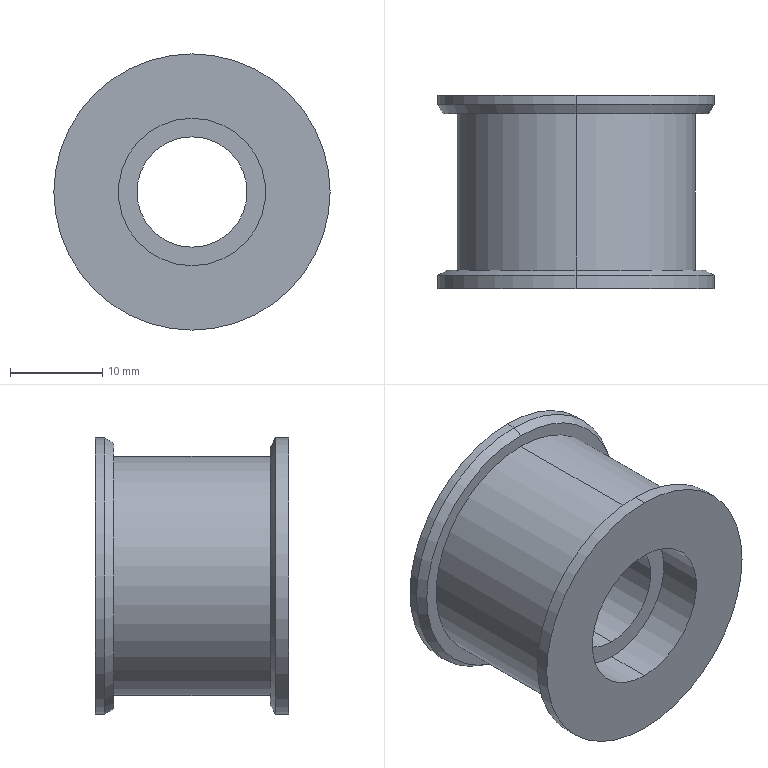Part | SolidWorks | features Chamfer 2, ICE 2, MirrorPattern 1, Revolution 1 | 1 solid | 22 faces | box 30 x 21 x 30 mm | volume 8531 mm3 | cylinder 12 | plane 6 | cone 4 | commonest cylinder face diameters 16 x4 30 x4 12 x2 25.98 x2
STEP:
#1=CARTESIAN_POINT('',(0.,-8.5,14.));
#2=VERTEX_POINT('',#1);
#3=CARTESIAN_POINT('',(0.,-8.5,-14.));
#4=VERTEX_POINT('',#3);
#5=CARTESIAN_POINT('',(0.,-8.5,0.));
#6=DIRECTION('',(0.,1.,0.));
#7=DIRECTION('',(0.,0.,-1.));
#8=AXIS2_PLACEMENT_3D('',#5,#6,#7);
#9=CIRCLE('',#8,14.);
#10=EDGE_CURVE('',#2,#4,#9,.T.);
#11=ORIENTED_EDGE('',*,*,#10,.F.);
#12=CARTESIAN_POINT('',(0.,-9.077,15.));
#13=VERTEX_POINT('',#12);
#14=CARTESIAN_POINT('',(0.,-9.077,15.));
#15=DIRECTION('',(0.,-0.5,0.866));
#16=VECTOR('',#15,1000.);
#17=LINE('',#14,#16);
#18=EDGE_CURVE('',#2,#13,#17,.T.);
#19=ORIENTED_EDGE('',*,*,#18,.T.);
#20=CARTESIAN_POINT('',(0.,-9.077,-15.));
#21=VERTEX_POINT('',#20);
#22=CARTESIAN_POINT('',(0.,-9.077,0.));
#23=DIRECTION('',(0.,-1.,0.));
#24=DIRECTION('',(0.,0.,-1.));
#25=AXIS2_PLACEMENT_3D('',#22,#23,#24);
#26=CIRCLE('',#25,15.);
#27=EDGE_CURVE('',#21,#13,#26,.T.);
#28=ORIENTED_EDGE('',*,*,#27,.F.);
#29=CARTESIAN_POINT('',(0.,-9.077,-15.));
#30=DIRECTION('',(0.,-0.5,-0.866));
#31=VECTOR('',#30,1000.);
#32=LINE('',#29,#31);
#33=EDGE_CURVE('',#4,#21,#32,.T.);
#34=ORIENTED_EDGE('',*,*,#33,.F.);
#35=EDGE_LOOP('',(#11,#19,#28,#34));
#36=FACE_OUTER_BOUND('',#35,.T.);
#37=CARTESIAN_POINT('',(0.,-9.077,0.));
#38=DIRECTION('',(0.,-1.,0.));
#39=DIRECTION('',(0.,0.,-1.));
#40=AXIS2_PLACEMENT_3D('',#37,#38,#39);
#41=CONICAL_SURFACE('',#40,15.,1.047);
#42=ADVANCED_FACE('',(#36),#41,.T.);
#43=CARTESIAN_POINT('',(0.,8.5,-14.423));
#44=VERTEX_POINT('',#43);
#45=CARTESIAN_POINT('',(0.,8.5,14.423));
#46=VERTEX_POINT('',#45);
#47=CARTESIAN_POINT('',(0.,8.5,0.));
#48=DIRECTION('',(0.,-1.,0.));
#49=DIRECTION('',(0.,0.,1.));
#50=AXIS2_PLACEMENT_3D('',#47,#48,#49);
#51=CIRCLE('',#50,14.423);
#52=EDGE_CURVE('',#44,#46,#51,.T.);
#53=ORIENTED_EDGE('',*,*,#52,.F.);
#54=CARTESIAN_POINT('',(0.,9.5,-15.));
#55=VERTEX_POINT('',#54);
#56=CARTESIAN_POINT('',(0.,8.5,-14.423));
#57=DIRECTION('',(0.,0.866,-0.5));
#58=VECTOR('',#57,1000.);
#59=LINE('',#56,#58);
#60=EDGE_CURVE('',#44,#55,#59,.T.);
#61=ORIENTED_EDGE('',*,*,#60,.T.);
#62=CARTESIAN_POINT('',(0.,9.5,15.));
#63=VERTEX_POINT('',#62);
#64=CARTESIAN_POINT('',(0.,9.5,0.));
#65=DIRECTION('',(0.,1.,0.));
#66=DIRECTION('',(0.,0.,1.));
#67=AXIS2_PLACEMENT_3D('',#64,#65,#66);
#68=CIRCLE('',#67,15.);
#69=EDGE_CURVE('',#63,#55,#68,.T.);
#70=ORIENTED_EDGE('',*,*,#69,.F.);
#71=CARTESIAN_POINT('',(0.,8.5,14.423));
#72=DIRECTION('',(0.,0.866,0.5));
#73=VECTOR('',#72,1000.);
#74=LINE('',#71,#73);
#75=EDGE_CURVE('',#46,#63,#74,.T.);
#76=ORIENTED_EDGE('',*,*,#75,.F.);
#77=EDGE_LOOP('',(#53,#61,#70,#76));
#78=FACE_OUTER_BOUND('',#77,.T.);
#79=CARTESIAN_POINT('',(0.,8.5,0.));
#80=DIRECTION('',(0.,1.,0.));
#81=DIRECTION('',(0.,0.,1.));
#82=AXIS2_PLACEMENT_3D('',#79,#80,#81);
#83=CONICAL_SURFACE('',#82,14.423,0.5236);
#84=ADVANCED_FACE('',(#78),#83,.T.);
#85=ORIENTED_EDGE('',*,*,#69,.T.);
#86=CARTESIAN_POINT('',(0.,10.5,-15.));
#87=VERTEX_POINT('',#86);
#88=CARTESIAN_POINT('',(0.,8.5,-15.));
#89=DIRECTION('',(0.,1.,0.));
#90=VECTOR('',#89,1000.);
#91=LINE('',#88,#90);
#92=EDGE_CURVE('',#55,#87,#91,.T.);
#93=ORIENTED_EDGE('',*,*,#92,.T.);
#94=CARTESIAN_POINT('',(0.,10.5,15.));
#95=VERTEX_POINT('',#94);
#96=CARTESIAN_POINT('',(0.,10.5,0.));
#97=DIRECTION('',(0.,-1.,0.));
#98=DIRECTION('',(0.,0.,-1.));
#99=AXIS2_PLACEMENT_3D('',#96,#97,#98);
#100=CIRCLE('',#99,15.);
#101=EDGE_CURVE('',#87,#95,#100,.T.);
#102=ORIENTED_EDGE('',*,*,#101,.T.);
#103=CARTESIAN_POINT('',(0.,8.5,15.));
#104=DIRECTION('',(0.,1.,0.));
#105=VECTOR('',#104,1000.);
#106=LINE('',#103,#105);
#107=EDGE_CURVE('',#63,#95,#106,.T.);
#108=ORIENTED_EDGE('',*,*,#107,.F.);
#109=EDGE_LOOP('',(#85,#93,#102,#108));
#110=FACE_OUTER_BOUND('',#109,.T.);
#111=CARTESIAN_POINT('',(0.,8.5,0.));
#112=DIRECTION('',(0.,1.,0.));
#113=DIRECTION('',(0.,0.,1.));
#114=AXIS2_PLACEMENT_3D('',#111,#112,#113);
#115=CYLINDRICAL_SURFACE('',#114,15.);
#116=ADVANCED_FACE('',(#110),#115,.T.);
#117=CARTESIAN_POINT('',(0.,5.5,8.));
#118=VERTEX_POINT('',#117);
#119=CARTESIAN_POINT('',(0.,5.5,-8.));
#120=VERTEX_POINT('',#119);
#121=CARTESIAN_POINT('',(0.,5.5,0.));
#122=DIRECTION('',(0.,-1.,0.));
#123=DIRECTION('',(0.,0.,-1.));
#124=AXIS2_PLACEMENT_3D('',#121,#122,#123);
#125=CIRCLE('',#124,8.);
#126=EDGE_CURVE('',#118,#120,#125,.T.);
#127=ORIENTED_EDGE('',*,*,#126,.T.);
#128=CARTESIAN_POINT('',(0.,10.5,-8.));
#129=VERTEX_POINT('',#128);
#130=CARTESIAN_POINT('',(0.,5.5,-8.));
#131=DIRECTION('',(0.,1.,0.));
#132=VECTOR('',#131,1000.);
#133=LINE('',#130,#132);
#134=EDGE_CURVE('',#120,#129,#133,.T.);
#135=ORIENTED_EDGE('',*,*,#134,.T.);
#136=CARTESIAN_POINT('',(0.,10.5,8.));
#137=VERTEX_POINT('',#136);
#138=CARTESIAN_POINT('',(0.,10.5,0.));
#139=DIRECTION('',(0.,-1.,0.));
#140=DIRECTION('',(0.,0.,-1.));
#141=AXIS2_PLACEMENT_3D('',#138,#139,#140);
#142=CIRCLE('',#141,8.);
#143=EDGE_CURVE('',#137,#129,#142,.T.);
#144=ORIENTED_EDGE('',*,*,#143,.F.);
#145=CARTESIAN_POINT('',(0.,5.5,8.));
#146=DIRECTION('',(0.,1.,0.));
#147=VECTOR('',#146,1000.);
#148=LINE('',#145,#147);
#149=EDGE_CURVE('',#118,#137,#148,.T.);
#150=ORIENTED_EDGE('',*,*,#149,.F.);
#151=EDGE_LOOP('',(#127,#135,#144,#150));
#152=FACE_OUTER_BOUND('',#151,.T.);
#153=CARTESIAN_POINT('',(0.,5.5,0.));
#154=DIRECTION('',(0.,1.,0.));
#155=DIRECTION('',(0.,0.,1.));
#156=AXIS2_PLACEMENT_3D('',#153,#154,#155);
#157=CYLINDRICAL_SURFACE('',#156,8.);
#158=ADVANCED_FACE('',(#152),#157,.F.);
#159=ORIENTED_EDGE('',*,*,#27,.T.);
#160=CARTESIAN_POINT('',(0.,-10.5,15.));
#161=VERTEX_POINT('',#160);
#162=CARTESIAN_POINT('',(0.,-8.5,15.));
#163=DIRECTION('',(0.,-1.,0.));
#164=VECTOR('',#163,1000.);
#165=LINE('',#162,#164);
#166=EDGE_CURVE('',#13,#161,#165,.T.);
#167=ORIENTED_EDGE('',*,*,#166,.T.);
#168=CARTESIAN_POINT('',(0.,-10.5,-15.));
#169=VERTEX_POINT('',#168);
#170=CARTESIAN_POINT('',(0.,-10.5,0.));
#171=DIRECTION('',(0.,-1.,0.));
#172=DIRECTION('',(0.,0.,-1.));
#173=AXIS2_PLACEMENT_3D('',#170,#171,#172);
#174=CIRCLE('',#173,15.);
#175=EDGE_CURVE('',#169,#161,#174,.T.);
#176=ORIENTED_EDGE('',*,*,#175,.F.);
#177=CARTESIAN_POINT('',(0.,-8.5,-15.));
#178=DIRECTION('',(0.,-1.,0.));
#179=VECTOR('',#178,1000.);
#180=LINE('',#177,#179);
#181=EDGE_CURVE('',#21,#169,#180,.T.);
#182=ORIENTED_EDGE('',*,*,#181,.F.);
#183=EDGE_LOOP('',(#159,#167,#176,#182));
#184=FACE_OUTER_BOUND('',#183,.T.);
#185=CARTESIAN_POINT('',(0.,-8.5,0.));
#186=DIRECTION('',(0.,-1.,0.));
#187=DIRECTION('',(0.,0.,-1.));
#188=AXIS2_PLACEMENT_3D('',#185,#186,#187);
#189=CYLINDRICAL_SURFACE('',#188,15.);
#190=ADVANCED_FACE('',(#184),#189,.T.);
#191=CARTESIAN_POINT('',(0.,-5.5,8.));
#192=VERTEX_POINT('',#191);
#193=CARTESIAN_POINT('',(0.,-5.5,-8.));
#194=VERTEX_POINT('',#193);
#195=CARTESIAN_POINT('',(0.,-5.5,0.));
#196=DIRECTION('',(0.,-1.,0.));
#197=DIRECTION('',(0.,0.,-1.));
#198=AXIS2_PLACEMENT_3D('',#195,#196,#197);
#199=CIRCLE('',#198,8.);
#200=EDGE_CURVE('',#192,#194,#199,.T.);
#201=ORIENTED_EDGE('',*,*,#200,.F.);
#202=CARTESIAN_POINT('',(0.,-10.5,8.));
#203=VERTEX_POINT('',#202);
#204=CARTESIAN_POINT('',(0.,-5.5,8.));
#205=DIRECTION('',(0.,-1.,0.));
#206=VECTOR('',#205,1000.);
#207=LINE('',#204,#206);
#208=EDGE_CURVE('',#192,#203,#207,.T.);
#209=ORIENTED_EDGE('',*,*,#208,.T.);
#210=CARTESIAN_POINT('',(0.,-10.5,-8.));
#211=VERTEX_POINT('',#210);
#212=CARTESIAN_POINT('',(0.,-10.5,0.));
#213=DIRECTION('',(0.,-1.,0.));
#214=DIRECTION('',(0.,0.,-1.));
#215=AXIS2_PLACEMENT_3D('',#212,#213,#214);
#216=CIRCLE('',#215,8.);
#217=EDGE_CURVE('',#203,#211,#216,.T.);
#218=ORIENTED_EDGE('',*,*,#217,.T.);
#219=CARTESIAN_POINT('',(0.,-5.5,-8.));
#220=DIRECTION('',(0.,-1.,0.));
#221=VECTOR('',#220,1000.);
#222=LINE('',#219,#221);
#223=EDGE_CURVE('',#194,#211,#222,.T.);
#224=ORIENTED_EDGE('',*,*,#223,.F.);
#225=EDGE_LOOP('',(#201,#209,#218,#224));
#226=FACE_OUTER_BOUND('',#225,.T.);
#227=CARTESIAN_POINT('',(0.,-5.5,0.));
#228=DIRECTION('',(0.,-1.,0.));
#229=DIRECTION('',(0.,0.,-1.));
#230=AXIS2_PLACEMENT_3D('',#227,#228,#229);
#231=CYLINDRICAL_SURFACE('',#230,8.);
#232=ADVANCED_FACE('',(#226),#231,.F.);
#233=CARTESIAN_POINT('',(0.,5.5,-6.));
#234=VERTEX_POINT('',#233);
#235=CARTESIAN_POINT('',(0.,5.5,6.));
#236=VERTEX_POINT('',#235);
#237=CARTESIAN_POINT('',(0.,5.5,0.));
#238=DIRECTION('',(0.,1.,0.));
#239=DIRECTION('',(0.,0.,1.));
#240=AXIS2_PLACEMENT_3D('',#237,#238,#239);
#241=CIRCLE('',#240,6.);
#242=EDGE_CURVE('',#234,#236,#241,.T.);
#243=ORIENTED_EDGE('',*,*,#242,.T.);
#244=CARTESIAN_POINT('',(0.,-5.5,6.));
#245=VERTEX_POINT('',#244);
#246=CARTESIAN_POINT('',(0.,0.,6.));
#247=DIRECTION('',(0.,-1.,0.));
#248=VECTOR('',#247,1000.);
#249=LINE('',#246,#248);
#250=EDGE_CURVE('',#236,#245,#249,.T.);
#251=ORIENTED_EDGE('',*,*,#250,.T.);
#252=CARTESIAN_POINT('',(0.,-5.5,-6.));
#253=VERTEX_POINT('',#252);
#254=CARTESIAN_POINT('',(0.,-5.5,0.));
#255=DIRECTION('',(0.,-1.,0.));
#256=DIRECTION('',(0.,0.,-1.));
#257=AXIS2_PLACEMENT_3D('',#254,#255,#256);
#258=CIRCLE('',#257,6.);
#259=EDGE_CURVE('',#245,#253,#258,.T.);
#260=ORIENTED_EDGE('',*,*,#259,.T.);
#261=CARTESIAN_POINT('',(0.,0.,-6.));
#262=DIRECTION('',(0.,-1.,0.));
#263=VECTOR('',#262,1000.);
#264=LINE('',#261,#263);
#265=EDGE_CURVE('',#234,#253,#264,.T.);
#266=ORIENTED_EDGE('',*,*,#265,.F.);
#267=EDGE_LOOP('',(#243,#251,#260,#266));
#268=FACE_OUTER_BOUND('',#267,.T.);
#269=CARTESIAN_POINT('',(0.,0.,0.));
#270=DIRECTION('',(0.,-1.,0.));
#271=DIRECTION('',(0.,0.,-1.));
#272=AXIS2_PLACEMENT_3D('',#269,#270,#271);
#273=CYLINDRICAL_SURFACE('',#272,6.);
#274=ADVANCED_FACE('',(#268),#273,.F.);
#275=CARTESIAN_POINT('',(0.,8.5,-12.99));
#276=VERTEX_POINT('',#275);
#277=CARTESIAN_POINT('',(0.,8.5,12.99));
#278=VERTEX_POINT('',#277);
#279=CARTESIAN_POINT('',(0.,8.5,0.));
#280=DIRECTION('',(0.,-1.,0.));
#281=DIRECTION('',(0.,0.,1.));
#282=AXIS2_PLACEMENT_3D('',#279,#280,#281);
#283=CIRCLE('',#282,12.99);
#284=EDGE_CURVE('',#276,#278,#283,.T.);
#285=ORIENTED_EDGE('',*,*,#284,.T.);
#286=CARTESIAN_POINT('',(0.,-8.5,12.99));
#287=VERTEX_POINT('',#286);
#288=CARTESIAN_POINT('',(0.,0.,12.99));
#289=DIRECTION('',(0.,-1.,0.));
#290=VECTOR('',#289,1000.);
#291=LINE('',#288,#290);
#292=EDGE_CURVE('',#278,#287,#291,.T.);
#293=ORIENTED_EDGE('',*,*,#292,.T.);
#294=CARTESIAN_POINT('',(0.,-8.5,-12.99));
#295=VERTEX_POINT('',#294);
#296=CARTESIAN_POINT('',(0.,-8.5,0.));
#297=DIRECTION('',(0.,1.,0.));
#298=DIRECTION('',(0.,0.,-1.));
#299=AXIS2_PLACEMENT_3D('',#296,#297,#298);
#300=CIRCLE('',#299,12.99);
#301=EDGE_CURVE('',#287,#295,#300,.T.);
#302=ORIENTED_EDGE('',*,*,#301,.T.);
#303=CARTESIAN_POINT('',(0.,0.,-12.99));
#304=DIRECTION('',(0.,-1.,0.));
#305=VECTOR('',#304,1000.);
#306=LINE('',#303,#305);
#307=EDGE_CURVE('',#276,#295,#306,.T.);
#308=ORIENTED_EDGE('',*,*,#307,.F.);
#309=EDGE_LOOP('',(#285,#293,#302,#308));
#310=FACE_OUTER_BOUND('',#309,.T.);
#311=CARTESIAN_POINT('',(0.,0.,0.));
#312=DIRECTION('',(0.,-1.,0.));
#313=DIRECTION('',(0.,0.,-1.));
#314=AXIS2_PLACEMENT_3D('',#311,#312,#313);
#315=CYLINDRICAL_SURFACE('',#314,12.99);
#316=ADVANCED_FACE('',(#310),#315,.T.);
#317=ORIENTED_EDGE('',*,*,#292,.F.);
#318=CARTESIAN_POINT('',(0.,8.5,0.));
#319=DIRECTION('',(0.,-1.,0.));
#320=DIRECTION('',(0.,0.,1.));
#321=AXIS2_PLACEMENT_3D('',#318,#319,#320);
#322=CIRCLE('',#321,12.99);
#323=EDGE_CURVE('',#278,#276,#322,.T.);
#324=ORIENTED_EDGE('',*,*,#323,.T.);
#325=ORIENTED_EDGE('',*,*,#307,.T.);
#326=CARTESIAN_POINT('',(0.,-8.5,0.));
#327=DIRECTION('',(0.,1.,0.));
#328=DIRECTION('',(0.,0.,-1.));
#329=AXIS2_PLACEMENT_3D('',#326,#327,#328);
#330=CIRCLE('',#329,12.99);
#331=EDGE_CURVE('',#295,#287,#330,.T.);
#332=ORIENTED_EDGE('',*,*,#331,.T.);
#333=EDGE_LOOP('',(#317,#324,#325,#332));
#334=FACE_OUTER_BOUND('',#333,.T.);
#335=CARTESIAN_POINT('',(0.,0.,0.));
#336=DIRECTION('',(0.,-1.,0.));
#337=DIRECTION('',(0.,0.,-1.));
#338=AXIS2_PLACEMENT_3D('',#335,#336,#337);
#339=CYLINDRICAL_SURFACE('',#338,12.99);
#340=ADVANCED_FACE('',(#334),#339,.T.);
#341=ORIENTED_EDGE('',*,*,#250,.F.);
#342=CARTESIAN_POINT('',(0.,5.5,0.));
#343=DIRECTION('',(0.,1.,0.));
#344=DIRECTION('',(0.,0.,1.));
#345=AXIS2_PLACEMENT_3D('',#342,#343,#344);
#346=CIRCLE('',#345,6.);
#347=EDGE_CURVE('',#236,#234,#346,.T.);
#348=ORIENTED_EDGE('',*,*,#347,.T.);
#349=ORIENTED_EDGE('',*,*,#265,.T.);
#350=CARTESIAN_POINT('',(0.,-5.5,0.));
#351=DIRECTION('',(0.,-1.,0.));
#352=DIRECTION('',(0.,0.,-1.));
#353=AXIS2_PLACEMENT_3D('',#350,#351,#352);
#354=CIRCLE('',#353,6.);
#355=EDGE_CURVE('',#253,#245,#354,.T.);
#356=ORIENTED_EDGE('',*,*,#355,.T.);
#357=EDGE_LOOP('',(#341,#348,#349,#356));
#358=FACE_OUTER_BOUND('',#357,.T.);
#359=CARTESIAN_POINT('',(0.,0.,0.));
#360=DIRECTION('',(0.,-1.,0.));
#361=DIRECTION('',(0.,0.,-1.));
#362=AXIS2_PLACEMENT_3D('',#359,#360,#361);
#363=CYLINDRICAL_SURFACE('',#362,6.);
#364=ADVANCED_FACE('',(#358),#363,.F.);
#365=ORIENTED_EDGE('',*,*,#143,.T.);
#366=CARTESIAN_POINT('',(0.,10.5,0.));
#367=DIRECTION('',(0.,-1.,0.));
#368=DIRECTION('',(0.,0.,-1.));
#369=AXIS2_PLACEMENT_3D('',#366,#367,#368);
#370=CIRCLE('',#369,8.);
#371=EDGE_CURVE('',#129,#137,#370,.T.);
#372=ORIENTED_EDGE('',*,*,#371,.T.);
#373=EDGE_LOOP('',(#365,#372));
#374=FACE_BOUND('',#373,.T.);
#375=CARTESIAN_POINT('',(0.,10.5,0.));
#376=DIRECTION('',(0.,-1.,0.));
#377=DIRECTION('',(0.,0.,-1.));
#378=AXIS2_PLACEMENT_3D('',#375,#376,#377);
#379=CIRCLE('',#378,15.);
#380=EDGE_CURVE('',#95,#87,#379,.T.);
#381=ORIENTED_EDGE('',*,*,#380,.F.);
#382=ORIENTED_EDGE('',*,*,#101,.F.);
#383=EDGE_LOOP('',(#381,#382));
#384=FACE_OUTER_BOUND('',#383,.T.);
#385=CARTESIAN_POINT('',(6.,10.5,0.));
#386=DIRECTION('',(0.,1.,0.));
#387=DIRECTION('',(0.,0.,1.));
#388=AXIS2_PLACEMENT_3D('',#385,#386,#387);
#389=PLANE('',#388);
#390=ADVANCED_FACE('',(#374,#384),#389,.T.);
#391=CARTESIAN_POINT('',(0.,-10.5,0.));
#392=DIRECTION('',(0.,-1.,0.));
#393=DIRECTION('',(0.,0.,-1.));
#394=AXIS2_PLACEMENT_3D('',#391,#392,#393);
#395=CIRCLE('',#394,8.);
#396=EDGE_CURVE('',#211,#203,#395,.T.);
#397=ORIENTED_EDGE('',*,*,#396,.F.);
#398=ORIENTED_EDGE('',*,*,#217,.F.);
#399=EDGE_LOOP('',(#397,#398));
#400=FACE_BOUND('',#399,.T.);
#401=ORIENTED_EDGE('',*,*,#175,.T.);
#402=CARTESIAN_POINT('',(0.,-10.5,0.));
#403=DIRECTION('',(0.,-1.,0.));
#404=DIRECTION('',(0.,0.,-1.));
#405=AXIS2_PLACEMENT_3D('',#402,#403,#404);
#406=CIRCLE('',#405,15.);
#407=EDGE_CURVE('',#161,#169,#406,.T.);
#408=ORIENTED_EDGE('',*,*,#407,.T.);
#409=EDGE_LOOP('',(#401,#408));
#410=FACE_OUTER_BOUND('',#409,.T.);
#411=CARTESIAN_POINT('',(12.99,-10.5,0.));
#412=DIRECTION('',(0.,-1.,0.));
#413=DIRECTION('',(0.,0.,-1.));
#414=AXIS2_PLACEMENT_3D('',#411,#412,#413);
#415=PLANE('',#414);
#416=ADVANCED_FACE('',(#400,#410),#415,.T.);
#417=ORIENTED_EDGE('',*,*,#208,.F.);
#418=CARTESIAN_POINT('',(0.,-5.5,0.));
#419=DIRECTION('',(0.,-1.,0.));
#420=DIRECTION('',(0.,0.,-1.));
#421=AXIS2_PLACEMENT_3D('',#418,#419,#420);
#422=CIRCLE('',#421,8.);
#423=EDGE_CURVE('',#194,#192,#422,.T.);
#424=ORIENTED_EDGE('',*,*,#423,.F.);
#425=ORIENTED_EDGE('',*,*,#223,.T.);
#426=ORIENTED_EDGE('',*,*,#396,.T.);
#427=EDGE_LOOP('',(#417,#424,#425,#426));
#428=FACE_OUTER_BOUND('',#427,.T.);
#429=CARTESIAN_POINT('',(0.,-5.5,0.));
#430=DIRECTION('',(0.,-1.,0.));
#431=DIRECTION('',(0.,0.,-1.));
#432=AXIS2_PLACEMENT_3D('',#429,#430,#431);
#433=CYLINDRICAL_SURFACE('',#432,8.);
#434=ADVANCED_FACE('',(#428),#433,.F.);
#435=ORIENTED_EDGE('',*,*,#355,.F.);
#436=ORIENTED_EDGE('',*,*,#259,.F.);
#437=EDGE_LOOP('',(#435,#436));
#438=FACE_BOUND('',#437,.T.);
#439=ORIENTED_EDGE('',*,*,#423,.T.);
#440=ORIENTED_EDGE('',*,*,#200,.T.);
#441=EDGE_LOOP('',(#439,#440));
#442=FACE_OUTER_BOUND('',#441,.T.);
#443=CARTESIAN_POINT('',(0.,-5.5,0.));
#444=DIRECTION('',(0.,-1.,0.));
#445=DIRECTION('',(0.,0.,-1.));
#446=AXIS2_PLACEMENT_3D('',#443,#444,#445);
#447=PLANE('',#446);
#448=ADVANCED_FACE('',(#438,#442),#447,.T.);
#449=ORIENTED_EDGE('',*,*,#166,.F.);
#450=CARTESIAN_POINT('',(0.,-9.077,0.));
#451=DIRECTION('',(0.,-1.,0.));
#452=DIRECTION('',(0.,0.,-1.));
#453=AXIS2_PLACEMENT_3D('',#450,#451,#452);
#454=CIRCLE('',#453,15.);
#455=EDGE_CURVE('',#13,#21,#454,.T.);
#456=ORIENTED_EDGE('',*,*,#455,.T.);
#457=ORIENTED_EDGE('',*,*,#181,.T.);
#458=ORIENTED_EDGE('',*,*,#407,.F.);
#459=EDGE_LOOP('',(#449,#456,#457,#458));
#460=FACE_OUTER_BOUND('',#459,.T.);
#461=CARTESIAN_POINT('',(0.,-8.5,0.));
#462=DIRECTION('',(0.,-1.,0.));
#463=DIRECTION('',(0.,0.,-1.));
#464=AXIS2_PLACEMENT_3D('',#461,#462,#463);
#465=CYLINDRICAL_SURFACE('',#464,15.);
#466=ADVANCED_FACE('',(#460),#465,.T.);
#467=CARTESIAN_POINT('',(0.,-8.5,0.));
#468=DIRECTION('',(0.,1.,0.));
#469=DIRECTION('',(0.,0.,-1.));
#470=AXIS2_PLACEMENT_3D('',#467,#468,#469);
#471=CIRCLE('',#470,14.);
#472=EDGE_CURVE('',#4,#2,#471,.T.);
#473=ORIENTED_EDGE('',*,*,#472,.T.);
#474=ORIENTED_EDGE('',*,*,#10,.T.);
#475=EDGE_LOOP('',(#473,#474));
#476=FACE_OUTER_BOUND('',#475,.T.);
#477=ORIENTED_EDGE('',*,*,#331,.F.);
#478=ORIENTED_EDGE('',*,*,#301,.F.);
#479=EDGE_LOOP('',(#477,#478));
#480=FACE_BOUND('',#479,.T.);
#481=CARTESIAN_POINT('',(0.,-8.5,0.));
#482=DIRECTION('',(0.,-1.,0.));
#483=DIRECTION('',(0.,0.,-1.));
#484=AXIS2_PLACEMENT_3D('',#481,#482,#483);
#485=PLANE('',#484);
#486=ADVANCED_FACE('',(#476,#480),#485,.F.);
#487=ORIENTED_EDGE('',*,*,#134,.F.);
#488=CARTESIAN_POINT('',(0.,5.5,0.));
#489=DIRECTION('',(0.,-1.,0.));
#490=DIRECTION('',(0.,0.,-1.));
#491=AXIS2_PLACEMENT_3D('',#488,#489,#490);
#492=CIRCLE('',#491,8.);
#493=EDGE_CURVE('',#120,#118,#492,.T.);
#494=ORIENTED_EDGE('',*,*,#493,.T.);
#495=ORIENTED_EDGE('',*,*,#149,.T.);
#496=ORIENTED_EDGE('',*,*,#371,.F.);
#497=EDGE_LOOP('',(#487,#494,#495,#496));
#498=FACE_OUTER_BOUND('',#497,.T.);
#499=CARTESIAN_POINT('',(0.,5.5,0.));
#500=DIRECTION('',(0.,1.,0.));
#501=DIRECTION('',(0.,0.,1.));
#502=AXIS2_PLACEMENT_3D('',#499,#500,#501);
#503=CYLINDRICAL_SURFACE('',#502,8.);
#504=ADVANCED_FACE('',(#498),#503,.F.);
#505=ORIENTED_EDGE('',*,*,#242,.F.);
#506=ORIENTED_EDGE('',*,*,#347,.F.);
#507=EDGE_LOOP('',(#505,#506));
#508=FACE_BOUND('',#507,.T.);
#509=ORIENTED_EDGE('',*,*,#126,.F.);
#510=ORIENTED_EDGE('',*,*,#493,.F.);
#511=EDGE_LOOP('',(#509,#510));
#512=FACE_OUTER_BOUND('',#511,.T.);
#513=CARTESIAN_POINT('',(0.,5.5,0.));
#514=DIRECTION('',(0.,1.,0.));
#515=DIRECTION('',(0.,0.,-1.));
#516=AXIS2_PLACEMENT_3D('',#513,#514,#515);
#517=PLANE('',#516);
#518=ADVANCED_FACE('',(#508,#512),#517,.T.);
#519=CARTESIAN_POINT('',(0.,8.5,0.));
#520=DIRECTION('',(0.,-1.,0.));
#521=DIRECTION('',(0.,0.,1.));
#522=AXIS2_PLACEMENT_3D('',#519,#520,#521);
#523=CIRCLE('',#522,14.423);
#524=EDGE_CURVE('',#46,#44,#523,.T.);
#525=ORIENTED_EDGE('',*,*,#524,.T.);
#526=ORIENTED_EDGE('',*,*,#52,.T.);
#527=EDGE_LOOP('',(#525,#526));
#528=FACE_OUTER_BOUND('',#527,.T.);
#529=ORIENTED_EDGE('',*,*,#284,.F.);
#530=ORIENTED_EDGE('',*,*,#323,.F.);
#531=EDGE_LOOP('',(#529,#530));
#532=FACE_BOUND('',#531,.T.);
#533=CARTESIAN_POINT('',(0.,8.5,0.));
#534=DIRECTION('',(0.,1.,0.));
#535=DIRECTION('',(0.,0.,-1.));
#536=AXIS2_PLACEMENT_3D('',#533,#534,#535);
#537=PLANE('',#536);
#538=ADVANCED_FACE('',(#528,#532),#537,.F.);
#539=ORIENTED_EDGE('',*,*,#92,.F.);
#540=CARTESIAN_POINT('',(0.,9.5,0.));
#541=DIRECTION('',(0.,1.,0.));
#542=DIRECTION('',(0.,0.,1.));
#543=AXIS2_PLACEMENT_3D('',#540,#541,#542);
#544=CIRCLE('',#543,15.);
#545=EDGE_CURVE('',#55,#63,#544,.T.);
#546=ORIENTED_EDGE('',*,*,#545,.T.);
#547=ORIENTED_EDGE('',*,*,#107,.T.);
#548=ORIENTED_EDGE('',*,*,#380,.T.);
#549=EDGE_LOOP('',(#539,#546,#547,#548));
#550=FACE_OUTER_BOUND('',#549,.T.);
#551=CARTESIAN_POINT('',(0.,8.5,0.));
#552=DIRECTION('',(0.,1.,0.));
#553=DIRECTION('',(0.,0.,1.));
#554=AXIS2_PLACEMENT_3D('',#551,#552,#553);
#555=CYLINDRICAL_SURFACE('',#554,15.);
#556=ADVANCED_FACE('',(#550),#555,.T.);
#557=ORIENTED_EDGE('',*,*,#60,.F.);
#558=ORIENTED_EDGE('',*,*,#524,.F.);
#559=ORIENTED_EDGE('',*,*,#75,.T.);
#560=ORIENTED_EDGE('',*,*,#545,.F.);
#561=EDGE_LOOP('',(#557,#558,#559,#560));
#562=FACE_OUTER_BOUND('',#561,.T.);
#563=CARTESIAN_POINT('',(0.,8.5,0.));
#564=DIRECTION('',(0.,1.,0.));
#565=DIRECTION('',(0.,0.,1.));
#566=AXIS2_PLACEMENT_3D('',#563,#564,#565);
#567=CONICAL_SURFACE('',#566,14.423,0.5236);
#568=ADVANCED_FACE('',(#562),#567,.T.);
#569=ORIENTED_EDGE('',*,*,#18,.F.);
#570=ORIENTED_EDGE('',*,*,#472,.F.);
#571=ORIENTED_EDGE('',*,*,#33,.T.);
#572=ORIENTED_EDGE('',*,*,#455,.F.);
#573=EDGE_LOOP('',(#569,#570,#571,#572));
#574=FACE_OUTER_BOUND('',#573,.T.);
#575=CARTESIAN_POINT('',(0.,-9.077,0.));
#576=DIRECTION('',(0.,-1.,0.));
#577=DIRECTION('',(0.,0.,-1.));
#578=AXIS2_PLACEMENT_3D('',#575,#576,#577);
#579=CONICAL_SURFACE('',#578,15.,1.047);
#580=ADVANCED_FACE('',(#574),#579,.T.);
#581=CLOSED_SHELL('',(#42,#84,#116,#158,#190,#232,#274,#316,#340,#364,#390,#416,#434,#448,#466,#486,#504,#518,#538,#556,#568,#580));
#582=MANIFOLD_SOLID_BREP('',#581);
#583=CARTESIAN_POINT('',(0.,0.,0.));
#584=DIRECTION('',(0.,0.,1.));
#585=DIRECTION('',(1.,0.,0.));
#586=AXIS2_PLACEMENT_3D('',#583,#584,#585);
#587=(LENGTH_UNIT()NAMED_UNIT(*)SI_UNIT(.MILLI.,.METRE.));
#588=UNCERTAINTY_MEASURE_WITH_UNIT(LENGTH_MEASURE(0.00001),#587,'','');
#589=(NAMED_UNIT(*)PLANE_ANGLE_UNIT()SI_UNIT($,.RADIAN.));
#590=(NAMED_UNIT(*)SI_UNIT($,.STERADIAN.)SOLID_ANGLE_UNIT());
#591=(GEOMETRIC_REPRESENTATION_CONTEXT(3)GLOBAL_UNCERTAINTY_ASSIGNED_CONTEXT((#588))GLOBAL_UNIT_ASSIGNED_CONTEXT((#587,#589,#590))REPRESENTATION_CONTEXT('',''));
#592=ADVANCED_BREP_SHAPE_REPRESENTATION('',(#582,#586),#591);